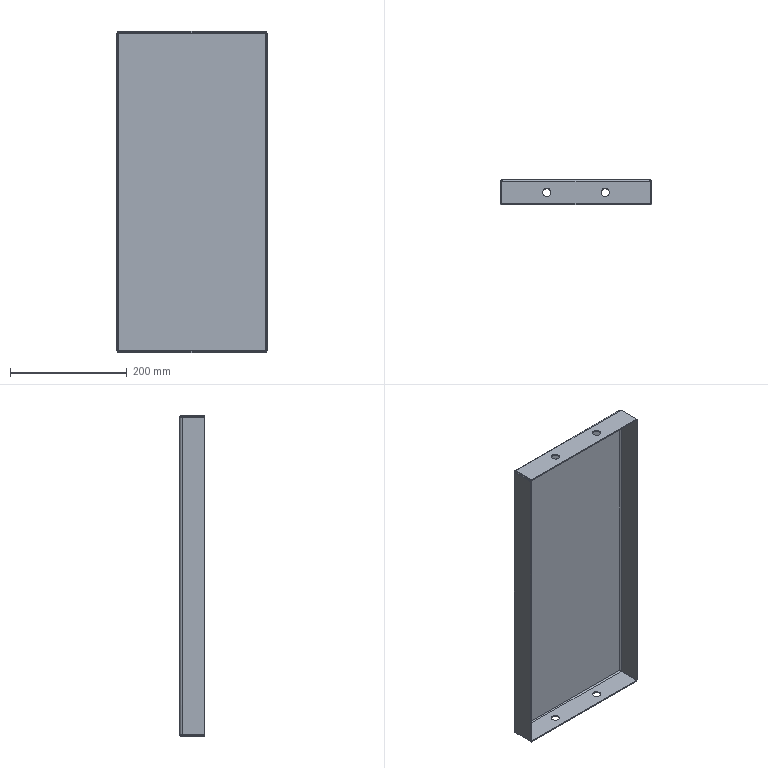Part | STEP file | Produce dryer line heating fan-OVEN-453 | 1 solid | 46 faces | box 260 x 42 x 550 mm | volume 408426 mm3 | plane 22 | cylinder 16 | spline 8 | commonest cylinder face diameters 14 x8 4 x4 8 x4